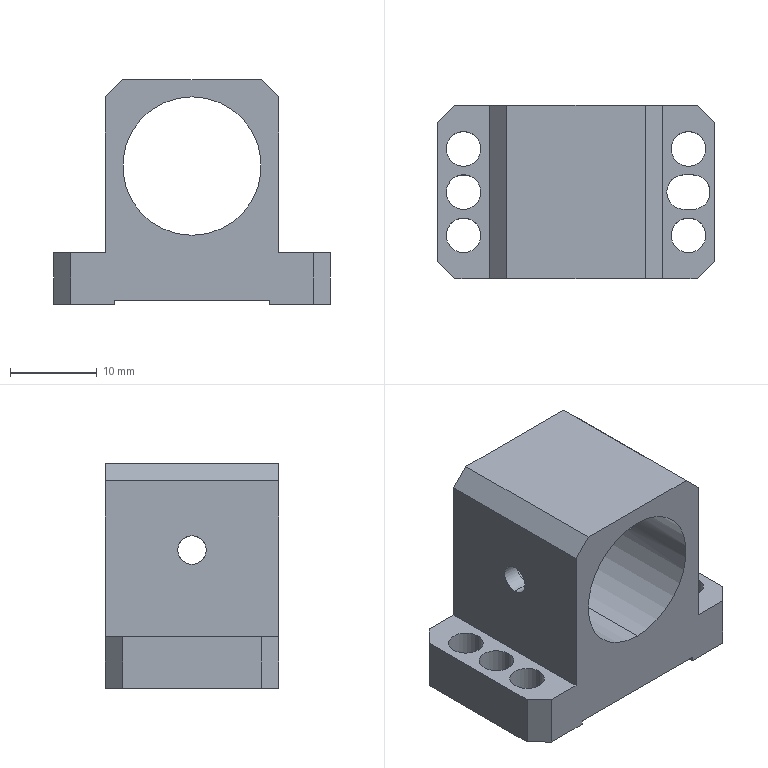NC program | NX | posted with a generic post | part box 32 x 20 x 26 mm
Lines 2180 to 2593 of 2593:
(ZLEVEL_PROFILE_1 , TOOL : D4R0.5)
N4334 T05 M6
N4336 G54
N4338 G17 G0 G90 X10.493 Y11.616 B0. C0. S9500 M3
N4340 G43 Z30. H5
N4342 Z0.929
N4344 G94 G1 Z-0.071 F1000.
N4346 X9.977 Y11.318
N4348 G3 X9.777 Y10.972 R0.4
N4350 G1 Y-10.972 F3000.
N4352 X9.813 Z-0.106
N4354 X9.848 Z-0.141
N4356 Y10.972
N4358 X9.884 Z-0.177
N4360 X9.919 Z-0.212
N4362 Y10.
N4364 Y-10.
N4366 Y-10.972
N4368 X9.955 Z-0.247
N4370 X9.989 Z-0.283
N4372 X9.99 Y-10.
N4374 Y10.
N4376 X9.989 Y10.972
N4378 X10.025 Z-0.318
N4380 X10.06 Z-0.354
N4382 X10.061 Y10.
N4384 Y-10.
N4386 X10.06 Y-10.972
N4388 X10.096 Z-0.389
N4390 X10.131 Z-0.424
N4392 Y-10.
N4394 Y10.
N4396 Y10.972
N4398 X10.167 Z-0.46
N4400 X10.202 Z-0.495
N4402 Y10.
N4404 Y-10.
N4406 Y-10.972
N4408 X10.237 Z-0.53
N4410 X10.272 Z-0.566
N4412 X10.273 Y-10.
N4414 Y10.
N4416 X10.272 Y10.972
N4418 X10.308 Y10.973 Z-0.601
N4420 X10.343 Z-0.636
N4422 X10.344 Y10.
N4424 Y-10.
N4426 X10.343 Y-10.973
N4428 X10.379 Z-0.672
N4430 X10.414 Z-0.707
N4432 Y-10.
N4434 Y10.
N4436 Y10.973
N4438 X10.45 Z-0.742
N4440 X10.484 Z-0.778
N4442 X10.485 Y10.
N4444 Y-10.
N4446 X10.484 Y-10.973
N4448 X10.52 Z-0.813
N4450 X10.555 Z-0.849
N4452 X10.556 Y-10.
N4454 Y10.
N4456 X10.555 Y10.973
N4458 X10.591 Z-0.884
N4460 X10.626 Z-0.919
N4462 Y10.
N4464 Y-10.
N4466 Y-10.973
N4468 X10.662 Z-0.955
N4470 X10.697 Z-0.99
N4472 Y-10.
N4474 Y10.
N4476 Y10.973
N4478 X10.732 Z-1.025
N4480 X10.767 Z-1.061
N4482 X10.768 Y10.
N4484 Y-10.
N4486 X10.767 Y-10.973
N4488 X10.803 Z-1.096
N4490 X10.838 Z-1.131
N4492 Y-10.
N4494 Y10.
N4496 Y10.973
N4498 X10.874 Z-1.167
N4500 X10.909 Z-1.202
N4502 Y10.
N4504 Y-10.
N4506 Y-10.973
N4508 X10.945 Z-1.237
N4510 X10.979 Z-1.273
N4512 X10.98 Y-10.
N4514 Y10.
N4516 X10.979 Y10.973
N4518 X11.015 Z-1.308
N4520 X11.05 Z-1.344
N4522 X11.051 Y10.
N4524 Y-10.
N4526 X11.05 Y-10.973
N4528 X11.086 Z-1.379
N4530 X11.121 Z-1.414
N4532 Y-10.
N4534 Y10.
N4536 Y10.973
N4538 X11.157 Z-1.45
N4540 X11.191 Z-1.485
N4542 X11.192 Y10.
N4544 Y-10.
N4546 X11.191 Y-10.973
N4548 X11.227 Z-1.52
N4550 X11.262 Z-1.556
N4552 X11.263 Y-10.
N4554 Y10.
N4556 X11.262 Y10.973
N4558 X11.298 Z-1.591
N4560 X11.333 Z-1.626
N4562 Y10.
N4564 Y-10.
N4566 Y-10.973
N4568 X11.369 Z-1.662
N4570 X11.404 Z-1.697
N4572 Y-10.
N4574 Y10.
N4576 Y10.972
N4578 X11.44 Z-1.732
N4580 X11.474 Z-1.768
N4582 X11.475 Y10.
N4584 Y-10.
N4586 X11.474 Y-10.972
N4588 X11.51 Z-1.803
N4590 X11.545 Z-1.838
N4592 X11.546 Y-10.
N4594 Y10.
N4596 X11.545 Y10.972
N4598 X11.581 Z-1.874
N4600 X11.616 Z-1.909
N4602 Y10.
N4604 Y-10.
N4606 Y-10.972
N4608 X11.652 Z-1.945
N4610 X11.686 Z-1.98
N4612 X11.687 Y-10.
N4614 Y10.
N4616 X11.686 Y10.972
N4618 X11.722 Z-2.015
N4620 X11.757 Z-2.051
N4622 X11.758 Y10.
N4624 Y-10.
N4626 X11.757 Y-10.972
N4628 X11.793 Z-2.086
N4630 X11.828 Z-2.121
N4632 Y-10.
N4634 Y10.
N4636 Y10.972
N4638 X11.864 Z-2.157
N4640 X11.899 Z-2.192
N4642 Y-10.972
N4644 X11.934 Z-2.227
N4646 X11.969 Z-2.263
N4648 Y10.972
N4650 X12. Z-2.292
N4652 X12.029 Z-2.322
N4654 Y-10.972
N4656 X12.059 Z-2.352
N4658 X12.088 Z-2.381
N4660 Y10.972
N4662 X12.118 Z-2.411
N4664 X12.147 Y10.971 Z-2.441
N4666 Y-10.972
N4668 X12.177 Z-2.47
N4670 X12.207 Z-2.5
N4672 Y10.971
N4674 G2 X12.407 Y11.318 R0.4
N4676 G1 X12.926 Y11.618
N4678 Z-1.5
N4680 G0 Z30.
N4682 X-10.493 Y-11.616
N4684 Z0.929
N4686 G1 Z-0.071 F1000.
N4688 X-9.977 Y-11.318
N4690 G3 X-9.777 Y-10.972 R0.4
N4692 G1 Y10.972 F3000.
N4694 X-9.813 Z-0.106
N4696 X-9.848 Z-0.141
N4698 Y-10.972
N4700 X-9.884 Z-0.177
N4702 X-9.919 Z-0.212
N4704 Y-10.
N4706 Y10.
N4708 Y10.972
N4710 X-9.955 Z-0.247
N4712 X-9.989 Z-0.283
N4714 X-9.99 Y10.
N4716 Y-10.
N4718 X-9.989 Y-10.972
N4720 X-10.025 Z-0.318
N4722 X-10.06 Z-0.354
N4724 X-10.061 Y-10.
N4726 Y10.
N4728 X-10.06 Y10.972
N4730 X-10.096 Z-0.389
N4732 X-10.131 Z-0.424
N4734 Y10.
N4736 Y-10.
N4738 Y-10.972
N4740 X-10.167 Z-0.46
N4742 X-10.202 Z-0.495
N4744 Y-10.
N4746 Y10.
N4748 Y10.972
N4750 X-10.237 Z-0.53
N4752 X-10.272 Z-0.566
N4754 X-10.273 Y10.
N4756 Y-10.
N4758 X-10.272 Y-10.972
N4760 X-10.308 Z-0.601
N4762 X-10.343 Y-10.973 Z-0.636
N4764 X-10.344 Y-10.
N4766 Y10.
N4768 X-10.343 Y10.973
N4770 X-10.379 Z-0.672
N4772 X-10.414 Z-0.707
N4774 Y10.
N4776 Y-10.
N4778 Y-10.973
N4780 X-10.45 Z-0.742
N4782 X-10.484 Z-0.778
N4784 X-10.485 Y-10.
N4786 Y10.
N4788 X-10.484 Y10.973
N4790 X-10.52 Z-0.813
N4792 X-10.555 Z-0.849
N4794 X-10.556 Y10.
N4796 Y-10.
N4798 X-10.555 Y-10.973
N4800 X-10.591 Z-0.884
N4802 X-10.626 Z-0.919
N4804 Y-10.
N4806 Y10.
N4808 Y10.973
N4810 X-10.662 Z-0.955
N4812 X-10.697 Z-0.99
N4814 Y10.
N4816 Y-10.
N4818 Y-10.973
N4820 X-10.732 Z-1.025
N4822 X-10.767 Z-1.061
N4824 X-10.768 Y-10.
N4826 Y10.
N4828 X-10.767 Y10.973
N4830 X-10.803 Z-1.096
N4832 X-10.838 Z-1.131
N4834 Y10.
N4836 Y-10.
N4838 Y-10.973
N4840 X-10.874 Z-1.167
N4842 X-10.909 Z-1.202
N4844 Y-10.
N4846 Y10.
N4848 Y10.973
N4850 X-10.945 Z-1.237
N4852 X-10.979 Z-1.273
N4854 X-10.98 Y10.
N4856 Y-10.
N4858 X-10.979 Y-10.973
N4860 X-11.015 Z-1.308
N4862 X-11.05 Z-1.344
N4864 X-11.051 Y-10.
N4866 Y10.
N4868 X-11.05 Y10.973
N4870 X-11.086 Z-1.379
N4872 X-11.121 Z-1.414
N4874 Y10.
N4876 Y-10.
N4878 Y-10.973
N4880 X-11.157 Z-1.45
N4882 X-11.191 Z-1.485
N4884 X-11.192 Y-10.
N4886 Y10.
N4888 X-11.191 Y10.973
N4890 X-11.227 Z-1.52
N4892 X-11.262 Z-1.556
N4894 X-11.263 Y10.
N4896 Y-10.
N4898 X-11.262 Y-10.973
N4900 X-11.298 Z-1.591
N4902 X-11.333 Z-1.626
N4904 Y-10.
N4906 Y10.
N4908 Y10.973
N4910 X-11.369 Z-1.662
N4912 X-11.404 Y10.972 Z-1.697
N4914 Y10.
N4916 Y-10.
N4918 Y-10.973
N4920 X-11.44 Y-10.972 Z-1.732
N4922 X-11.474 Z-1.768
N4924 X-11.475 Y-10.
N4926 Y10.
N4928 X-11.474 Y10.972
N4930 X-11.51 Z-1.803
N4932 X-11.545 Z-1.838
N4934 X-11.546 Y10.
N4936 Y-10.
N4938 X-11.545 Y-10.972
N4940 X-11.581 Z-1.874
N4942 X-11.616 Z-1.909
N4944 Y-10.
N4946 Y10.
N4948 Y10.972
N4950 X-11.652 Z-1.945
N4952 X-11.686 Z-1.98
N4954 X-11.687 Y10.
N4956 Y-10.
N4958 X-11.686 Y-10.972
N4960 X-11.722 Z-2.015
N4962 X-11.757 Z-2.051
N4964 X-11.758 Y-10.
N4966 Y10.
N4968 X-11.757 Y10.972
N4970 X-11.793 Z-2.086
N4972 X-11.828 Z-2.121
N4974 Y10.
N4976 Y-10.
N4978 Y-10.972
N4980 X-11.864 Z-2.157
N4982 X-11.899 Z-2.192
N4984 Y10.972
N4986 X-11.934 Z-2.227
N4988 X-11.969 Z-2.263
N4990 Y-10.972
N4992 X-12. Z-2.292
N4994 X-12.029 Z-2.322
N4996 Y10.972
N4998 X-12.059 Z-2.352
N5000 X-12.088 Z-2.381
N5002 Y-10.972
N5004 X-12.118 Z-2.411
N5006 X-12.147 Z-2.441
N5008 Y10.971
N5010 X-12.177 Z-2.47
N5012 X-12.207 Z-2.5
N5014 Y-10.972
N5016 G2 X-12.407 Y-11.318 R0.4
N5018 G1 X-12.926 Y-11.618
N5020 Z-1.5
N5022 G0 Z30.
N5024 M5
(PLANAR_MILL_COPY , TOOL : D6A45)
N5026 T07 M6
N5028 G54
N5030 G17 G0 G90 X-12. Y-1.27 B0. C0. S9500 M3
N5032 G43 Z30. H7
N5034 Z0.5
N5036 G94 G1 Z-1. F1250.
N5038 X-11.3 Y-0.866
N5040 G3 X-10.8 Y0. R1.
N5042 G1 Y9.8
N5044 G2 X-9.8 Y10.8 R1.
N5046 G1 X9.8
N5048 G2 X10.8 Y9.8 R1.
N5050 G1 Y-9.8
N5052 G2 X9.8 Y-10.8 R1.
N5054 G1 X-9.8
N5056 G2 X-10.8 Y-9.8 R1.
N5058 G1 Y0.
N5060 G3 X-11.3 Y0.866 R1.
N5062 G1 X-12. Y1.27
N5064 Z0.5
N5066 G0 Z30.
(PLANAR_MILL_COPY_COPY , TOOL : D6A45)
N5068 X14.158 Y12.191
N5070 Z-19.5
N5072 G1 Z-21.
N5074 X13.696 Y11.757
N5076 G3 X13.407 Y10.8 R1.
N5078 G1 X13.917
N5080 G2 X14.624 Y10.507 R1.
N5082 G1 X16.507 Y8.624
N5084 G2 X16.8 Y7.917 R1.
N5086 G1 Y-7.917
N5088 G2 X16.507 Y-8.624 R1.
N5090 G1 X14.624 Y-10.507
N5092 G2 X13.917 Y-10.8 R1.
N5094 G1 X13.407
N5096 G3 X13.696 Y-11.757 R1.
N5098 G1 X14.158 Y-12.191
N5100 Z-19.5
N5102 G0 Z30.
N5104 X-14.158
N5106 Z-19.5
N5108 G1 Z-21.
N5110 X-13.696 Y-11.757
N5112 G3 X-13.407 Y-10.8 R1.
N5114 G1 X-13.917
N5116 G2 X-14.624 Y-10.507 R1.
N5118 G1 X-16.507 Y-8.624
N5120 G2 X-16.8 Y-7.917 R1.
N5122 G1 Y7.917
N5124 G2 X-16.507 Y8.624 R1.
N5126 G1 X-14.624 Y10.507
N5128 G2 X-13.917 Y10.8 R1.
N5130 G1 X-13.407
N5132 G3 X-13.696 Y11.757 R1.
N5134 G1 X-14.158 Y12.191
N5136 Z-19.5
N5138 G0 Z30.
N5140 M5
N5142 M2